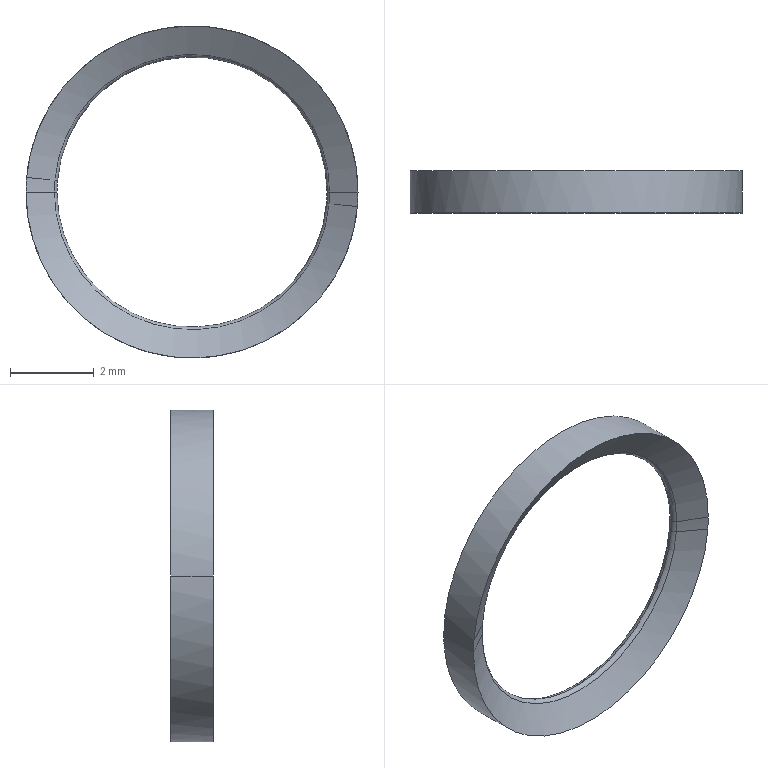Part | SolidWorks | features BaseBody 1 | 1 solid | 18 faces | box 7.92 x 1.004 x 7.92 mm | volume 9.83 mm3 | torus 8 | cone 8 | cylinder 2 | commonest cylinder face diameters 7.92 x2
STEP:
#1=CARTESIAN_POINT('',(-2079.52,1131.328,-1627.094));
#2=VERTEX_POINT('',#1);
#3=CARTESIAN_POINT('',(-2087.425,1131.328,-1627.439));
#4=VERTEX_POINT('',#3);
#5=CARTESIAN_POINT('',(-2083.48,1131.328,-1627.094));
#6=DIRECTION('',(0.,1.,0.));
#7=DIRECTION('',(1.,0.,0.));
#8=AXIS2_PLACEMENT_3D('',#5,#6,#7);
#9=CIRCLE('',#8,3.96);
#10=EDGE_CURVE('',#2,#4,#9,.T.);
#11=ORIENTED_EDGE('',*,*,#10,.F.);
#12=CARTESIAN_POINT('',(-2079.52,1130.324,-1627.094));
#13=VERTEX_POINT('',#12);
#14=CARTESIAN_POINT('',(-2079.52,1130.324,-1627.094));
#15=DIRECTION('',(0.,1.,0.));
#16=VECTOR('',#15,1000.);
#17=LINE('',#14,#16);
#18=EDGE_CURVE('',#13,#2,#17,.T.);
#19=ORIENTED_EDGE('',*,*,#18,.F.);
#20=CARTESIAN_POINT('',(-2079.536,1130.324,-1627.439));
#21=VERTEX_POINT('',#20);
#22=CARTESIAN_POINT('',(-2083.48,1130.324,-1627.094));
#23=DIRECTION('',(0.,1.,0.));
#24=DIRECTION('',(1.,0.,0.));
#25=AXIS2_PLACEMENT_3D('',#22,#23,#24);
#26=CIRCLE('',#25,3.96);
#27=EDGE_CURVE('',#13,#21,#26,.T.);
#28=ORIENTED_EDGE('',*,*,#27,.T.);
#29=CARTESIAN_POINT('',(-2087.44,1130.324,-1627.094));
#30=VERTEX_POINT('',#29);
#31=CARTESIAN_POINT('',(-2083.48,1130.324,-1627.094));
#32=DIRECTION('',(0.,1.,0.));
#33=DIRECTION('',(0.9962,0.,-0.08716));
#34=AXIS2_PLACEMENT_3D('',#31,#32,#33);
#35=CIRCLE('',#34,3.96);
#36=EDGE_CURVE('',#21,#30,#35,.T.);
#37=ORIENTED_EDGE('',*,*,#36,.T.);
#38=CARTESIAN_POINT('',(-2087.44,1131.328,-1627.094));
#39=VERTEX_POINT('',#38);
#40=CARTESIAN_POINT('',(-2087.44,1130.324,-1627.094));
#41=DIRECTION('',(0.,1.,0.));
#42=VECTOR('',#41,1000.);
#43=LINE('',#40,#42);
#44=EDGE_CURVE('',#30,#39,#43,.T.);
#45=ORIENTED_EDGE('',*,*,#44,.T.);
#46=CARTESIAN_POINT('',(-2083.48,1131.328,-1627.094));
#47=DIRECTION('',(0.,1.,0.));
#48=DIRECTION('',(-0.9962,0.,-0.08716));
#49=AXIS2_PLACEMENT_3D('',#46,#47,#48);
#50=CIRCLE('',#49,3.96);
#51=EDGE_CURVE('',#4,#39,#50,.T.);
#52=ORIENTED_EDGE('',*,*,#51,.F.);
#53=EDGE_LOOP('',(#11,#19,#28,#37,#45,#52));
#54=FACE_OUTER_BOUND('',#53,.T.);
#55=CARTESIAN_POINT('',(-2083.48,1124.59,-1627.094));
#56=DIRECTION('',(0.,1.,0.));
#57=DIRECTION('',(0.9962,0.,0.08716));
#58=AXIS2_PLACEMENT_3D('',#55,#56,#57);
#59=CYLINDRICAL_SURFACE('',#58,3.96);
#60=ADVANCED_FACE('',(#54),#59,.T.);
#61=CARTESIAN_POINT('',(-2087.425,1130.324,-1626.748));
#62=VERTEX_POINT('',#61);
#63=CARTESIAN_POINT('',(-2083.48,1130.324,-1627.094));
#64=DIRECTION('',(0.,1.,0.));
#65=DIRECTION('',(-0.9962,0.,0.08716));
#66=AXIS2_PLACEMENT_3D('',#63,#64,#65);
#67=CIRCLE('',#66,3.96);
#68=EDGE_CURVE('',#62,#13,#67,.T.);
#69=ORIENTED_EDGE('',*,*,#68,.T.);
#70=ORIENTED_EDGE('',*,*,#18,.T.);
#71=CARTESIAN_POINT('',(-2079.536,1131.328,-1626.748));
#72=VERTEX_POINT('',#71);
#73=CARTESIAN_POINT('',(-2083.48,1131.328,-1627.094));
#74=DIRECTION('',(0.,1.,0.));
#75=DIRECTION('',(0.9962,0.,0.08716));
#76=AXIS2_PLACEMENT_3D('',#73,#74,#75);
#77=CIRCLE('',#76,3.96);
#78=EDGE_CURVE('',#72,#2,#77,.T.);
#79=ORIENTED_EDGE('',*,*,#78,.F.);
#80=CARTESIAN_POINT('',(-2083.48,1131.328,-1627.094));
#81=DIRECTION('',(0.,1.,0.));
#82=DIRECTION('',(-1.,0.,0.));
#83=AXIS2_PLACEMENT_3D('',#80,#81,#82);
#84=CIRCLE('',#83,3.96);
#85=EDGE_CURVE('',#39,#72,#84,.T.);
#86=ORIENTED_EDGE('',*,*,#85,.F.);
#87=ORIENTED_EDGE('',*,*,#44,.F.);
#88=CARTESIAN_POINT('',(-2083.48,1130.324,-1627.094));
#89=DIRECTION('',(0.,1.,0.));
#90=DIRECTION('',(-1.,0.,0.));
#91=AXIS2_PLACEMENT_3D('',#88,#89,#90);
#92=CIRCLE('',#91,3.96);
#93=EDGE_CURVE('',#30,#62,#92,.T.);
#94=ORIENTED_EDGE('',*,*,#93,.T.);
#95=EDGE_LOOP('',(#69,#70,#79,#86,#87,#94));
#96=FACE_OUTER_BOUND('',#95,.T.);
#97=CARTESIAN_POINT('',(-2083.48,1124.59,-1627.094));
#98=DIRECTION('',(0.,1.,0.));
#99=DIRECTION('',(-0.9962,0.,-0.08716));
#100=AXIS2_PLACEMENT_3D('',#97,#98,#99);
#101=CYLINDRICAL_SURFACE('',#100,3.96);
#102=ADVANCED_FACE('',(#96),#101,.T.);
#103=CARTESIAN_POINT('',(-2080.207,1130.713,-1627.38));
#104=VERTEX_POINT('',#103);
#105=CARTESIAN_POINT('',(-2080.272,1130.826,-1627.374));
#106=VERTEX_POINT('',#105);
#107=CARTESIAN_POINT('',(-2080.143,1130.826,-1627.386));
#108=DIRECTION('',(-0.08716,0.,-0.9962));
#109=DIRECTION('',(-0.4981,-0.866,0.04358));
#110=AXIS2_PLACEMENT_3D('',#107,#108,#109);
#111=CIRCLE('',#110,0.1299);
#112=EDGE_CURVE('',#104,#106,#111,.T.);
#113=ORIENTED_EDGE('',*,*,#112,.T.);
#114=CARTESIAN_POINT('',(-2086.701,1130.826,-1627.094));
#115=VERTEX_POINT('',#114);
#116=CARTESIAN_POINT('',(-2083.48,1130.826,-1627.094));
#117=DIRECTION('',(0.,-1.,0.));
#118=DIRECTION('',(-1.,0.,0.));
#119=AXIS2_PLACEMENT_3D('',#116,#117,#118);
#120=CIRCLE('',#119,3.221);
#121=EDGE_CURVE('',#115,#106,#120,.T.);
#122=ORIENTED_EDGE('',*,*,#121,.F.);
#123=CARTESIAN_POINT('',(-2086.766,1130.713,-1627.094));
#124=VERTEX_POINT('',#123);
#125=CARTESIAN_POINT('',(-2086.831,1130.826,-1627.094));
#126=DIRECTION('',(0.,0.,1.));
#127=DIRECTION('',(0.5,-0.866,0.));
#128=AXIS2_PLACEMENT_3D('',#125,#126,#127);
#129=CIRCLE('',#128,0.1299);
#130=EDGE_CURVE('',#124,#115,#129,.T.);
#131=ORIENTED_EDGE('',*,*,#130,.F.);
#132=CARTESIAN_POINT('',(-2083.48,1130.713,-1627.094));
#133=DIRECTION('',(0.,-1.,0.));
#134=DIRECTION('',(-1.,0.,0.));
#135=AXIS2_PLACEMENT_3D('',#132,#133,#134);
#136=CIRCLE('',#135,3.286);
#137=EDGE_CURVE('',#124,#104,#136,.T.);
#138=ORIENTED_EDGE('',*,*,#137,.T.);
#139=EDGE_LOOP('',(#113,#122,#131,#138));
#140=FACE_OUTER_BOUND('',#139,.T.);
#141=CARTESIAN_POINT('',(-2083.48,1130.826,-1627.094));
#142=DIRECTION('',(0.,-1.,0.));
#143=DIRECTION('',(-0.9962,0.,0.08716));
#144=AXIS2_PLACEMENT_3D('',#141,#142,#143);
#145=TOROIDAL_SURFACE('',#144,3.35,0.1299);
#146=ADVANCED_FACE('',(#140),#145,.T.);
#147=CARTESIAN_POINT('',(-2086.754,1130.713,-1626.807));
#148=VERTEX_POINT('',#147);
#149=CARTESIAN_POINT('',(-2086.689,1130.826,-1626.813));
#150=VERTEX_POINT('',#149);
#151=CARTESIAN_POINT('',(-2086.818,1130.826,-1626.802));
#152=DIRECTION('',(0.08716,0.,0.9962));
#153=DIRECTION('',(0.4981,-0.866,-0.04358));
#154=AXIS2_PLACEMENT_3D('',#151,#152,#153);
#155=CIRCLE('',#154,0.1299);
#156=EDGE_CURVE('',#148,#150,#155,.T.);
#157=ORIENTED_EDGE('',*,*,#156,.T.);
#158=CARTESIAN_POINT('',(-2080.26,1130.826,-1627.094));
#159=VERTEX_POINT('',#158);
#160=CARTESIAN_POINT('',(-2083.48,1130.826,-1627.094));
#161=DIRECTION('',(0.,-1.,0.));
#162=DIRECTION('',(1.,0.,0.));
#163=AXIS2_PLACEMENT_3D('',#160,#161,#162);
#164=CIRCLE('',#163,3.221);
#165=EDGE_CURVE('',#159,#150,#164,.T.);
#166=ORIENTED_EDGE('',*,*,#165,.F.);
#167=CARTESIAN_POINT('',(-2080.195,1130.713,-1627.094));
#168=VERTEX_POINT('',#167);
#169=CARTESIAN_POINT('',(-2080.13,1130.826,-1627.094));
#170=DIRECTION('',(0.,0.,-1.));
#171=DIRECTION('',(-0.5,-0.866,0.));
#172=AXIS2_PLACEMENT_3D('',#169,#170,#171);
#173=CIRCLE('',#172,0.1299);
#174=EDGE_CURVE('',#168,#159,#173,.T.);
#175=ORIENTED_EDGE('',*,*,#174,.F.);
#176=CARTESIAN_POINT('',(-2083.48,1130.713,-1627.094));
#177=DIRECTION('',(0.,-1.,0.));
#178=DIRECTION('',(1.,0.,0.));
#179=AXIS2_PLACEMENT_3D('',#176,#177,#178);
#180=CIRCLE('',#179,3.286);
#181=EDGE_CURVE('',#168,#148,#180,.T.);
#182=ORIENTED_EDGE('',*,*,#181,.T.);
#183=EDGE_LOOP('',(#157,#166,#175,#182));
#184=FACE_OUTER_BOUND('',#183,.T.);
#185=CARTESIAN_POINT('',(-2083.48,1130.826,-1627.094));
#186=DIRECTION('',(0.,-1.,0.));
#187=DIRECTION('',(0.9962,0.,-0.08716));
#188=AXIS2_PLACEMENT_3D('',#185,#186,#187);
#189=TOROIDAL_SURFACE('',#188,3.35,0.1299);
#190=ADVANCED_FACE('',(#184),#189,.T.);
#191=CARTESIAN_POINT('',(-2086.754,1130.938,-1626.807));
#192=VERTEX_POINT('',#191);
#193=CARTESIAN_POINT('',(-2086.818,1130.826,-1626.802));
#194=DIRECTION('',(0.08716,0.,0.9962));
#195=DIRECTION('',(0.9962,0.,-0.08716));
#196=AXIS2_PLACEMENT_3D('',#193,#194,#195);
#197=CIRCLE('',#196,0.1299);
#198=EDGE_CURVE('',#150,#192,#197,.T.);
#199=ORIENTED_EDGE('',*,*,#198,.T.);
#200=CARTESIAN_POINT('',(-2080.207,1130.938,-1626.807));
#201=VERTEX_POINT('',#200);
#202=CARTESIAN_POINT('',(-2083.48,1130.938,-1627.094));
#203=DIRECTION('',(0.,-1.,0.));
#204=DIRECTION('',(0.9962,0.,0.08716));
#205=AXIS2_PLACEMENT_3D('',#202,#203,#204);
#206=CIRCLE('',#205,3.286);
#207=EDGE_CURVE('',#201,#192,#206,.T.);
#208=ORIENTED_EDGE('',*,*,#207,.F.);
#209=CARTESIAN_POINT('',(-2080.195,1130.938,-1627.094));
#210=VERTEX_POINT('',#209);
#211=CARTESIAN_POINT('',(-2083.48,1130.938,-1627.094));
#212=DIRECTION('',(0.,-1.,0.));
#213=DIRECTION('',(1.,0.,0.));
#214=AXIS2_PLACEMENT_3D('',#211,#212,#213);
#215=CIRCLE('',#214,3.286);
#216=EDGE_CURVE('',#210,#201,#215,.T.);
#217=ORIENTED_EDGE('',*,*,#216,.F.);
#218=CARTESIAN_POINT('',(-2080.13,1130.826,-1627.094));
#219=DIRECTION('',(0.,0.,-1.));
#220=DIRECTION('',(-1.,0.,0.));
#221=AXIS2_PLACEMENT_3D('',#218,#219,#220);
#222=CIRCLE('',#221,0.1299);
#223=EDGE_CURVE('',#159,#210,#222,.T.);
#224=ORIENTED_EDGE('',*,*,#223,.F.);
#225=ORIENTED_EDGE('',*,*,#165,.T.);
#226=EDGE_LOOP('',(#199,#208,#217,#224,#225));
#227=FACE_OUTER_BOUND('',#226,.T.);
#228=CARTESIAN_POINT('',(-2083.48,1130.826,-1627.094));
#229=DIRECTION('',(0.,-1.,0.));
#230=DIRECTION('',(0.9962,0.,-0.08716));
#231=AXIS2_PLACEMENT_3D('',#228,#229,#230);
#232=TOROIDAL_SURFACE('',#231,3.35,0.1299);
#233=ADVANCED_FACE('',(#227),#232,.T.);
#234=CARTESIAN_POINT('',(-2086.754,1130.938,-1627.38));
#235=VERTEX_POINT('',#234);
#236=CARTESIAN_POINT('',(-2087.425,1131.328,-1627.439));
#237=DIRECTION('',(0.8627,-0.5,0.07548));
#238=VECTOR('',#237,1000.);
#239=LINE('',#236,#238);
#240=EDGE_CURVE('',#4,#235,#239,.T.);
#241=ORIENTED_EDGE('',*,*,#240,.T.);
#242=CARTESIAN_POINT('',(-2080.207,1130.938,-1627.38));
#243=VERTEX_POINT('',#242);
#244=CARTESIAN_POINT('',(-2083.48,1130.938,-1627.094));
#245=DIRECTION('',(0.,-1.,0.));
#246=DIRECTION('',(-0.9962,0.,-0.08716));
#247=AXIS2_PLACEMENT_3D('',#244,#245,#246);
#248=CIRCLE('',#247,3.286);
#249=EDGE_CURVE('',#235,#243,#248,.T.);
#250=ORIENTED_EDGE('',*,*,#249,.T.);
#251=CARTESIAN_POINT('',(-2083.48,1130.938,-1627.094));
#252=DIRECTION('',(0.,-1.,0.));
#253=DIRECTION('',(0.9962,0.,-0.08716));
#254=AXIS2_PLACEMENT_3D('',#251,#252,#253);
#255=CIRCLE('',#254,3.286);
#256=EDGE_CURVE('',#243,#210,#255,.T.);
#257=ORIENTED_EDGE('',*,*,#256,.T.);
#258=CARTESIAN_POINT('',(-2080.195,1130.938,-1627.094));
#259=DIRECTION('',(0.866,0.5,0.));
#260=VECTOR('',#259,1000.);
#261=LINE('',#258,#260);
#262=EDGE_CURVE('',#210,#2,#261,.T.);
#263=ORIENTED_EDGE('',*,*,#262,.T.);
#264=ORIENTED_EDGE('',*,*,#10,.T.);
#265=EDGE_LOOP('',(#241,#250,#257,#263,#264));
#266=FACE_OUTER_BOUND('',#265,.T.);
#267=CARTESIAN_POINT('',(-2083.48,1130.918,-1627.094));
#268=DIRECTION('',(0.,1.,0.));
#269=DIRECTION('',(0.9962,0.,0.08716));
#270=AXIS2_PLACEMENT_3D('',#267,#268,#269);
#271=CONICAL_SURFACE('',#270,3.25,1.047);
#272=ADVANCED_FACE('',(#266),#271,.F.);
#273=CARTESIAN_POINT('',(-2079.536,1130.324,-1627.439));
#274=DIRECTION('',(-0.8627,0.5,0.07548));
#275=VECTOR('',#274,1000.);
#276=LINE('',#273,#275);
#277=EDGE_CURVE('',#21,#104,#276,.T.);
#278=ORIENTED_EDGE('',*,*,#277,.T.);
#279=ORIENTED_EDGE('',*,*,#137,.F.);
#280=CARTESIAN_POINT('',(-2086.766,1130.713,-1627.094));
#281=DIRECTION('',(-0.866,-0.5,0.));
#282=VECTOR('',#281,1000.);
#283=LINE('',#280,#282);
#284=EDGE_CURVE('',#124,#30,#283,.T.);
#285=ORIENTED_EDGE('',*,*,#284,.T.);
#286=ORIENTED_EDGE('',*,*,#36,.F.);
#287=EDGE_LOOP('',(#278,#279,#285,#286));
#288=FACE_OUTER_BOUND('',#287,.T.);
#289=CARTESIAN_POINT('',(-2083.48,1130.734,-1627.094));
#290=DIRECTION('',(0.,-1.,0.));
#291=DIRECTION('',(-0.9962,0.,0.08716));
#292=AXIS2_PLACEMENT_3D('',#289,#290,#291);
#293=CONICAL_SURFACE('',#292,3.25,1.047);
#294=ADVANCED_FACE('',(#288),#293,.F.);
#295=CARTESIAN_POINT('',(-2087.425,1130.324,-1626.748));
#296=DIRECTION('',(0.8627,0.5,-0.07548));
#297=VECTOR('',#296,1000.);
#298=LINE('',#295,#297);
#299=EDGE_CURVE('',#62,#148,#298,.T.);
#300=ORIENTED_EDGE('',*,*,#299,.T.);
#301=ORIENTED_EDGE('',*,*,#181,.F.);
#302=CARTESIAN_POINT('',(-2080.195,1130.713,-1627.094));
#303=DIRECTION('',(0.866,-0.5,0.));
#304=VECTOR('',#303,1000.);
#305=LINE('',#302,#304);
#306=EDGE_CURVE('',#168,#13,#305,.T.);
#307=ORIENTED_EDGE('',*,*,#306,.T.);
#308=ORIENTED_EDGE('',*,*,#68,.F.);
#309=EDGE_LOOP('',(#300,#301,#307,#308));
#310=FACE_OUTER_BOUND('',#309,.T.);
#311=CARTESIAN_POINT('',(-2083.48,1130.734,-1627.094));
#312=DIRECTION('',(0.,-1.,0.));
#313=DIRECTION('',(0.9962,0.,-0.08716));
#314=AXIS2_PLACEMENT_3D('',#311,#312,#313);
#315=CONICAL_SURFACE('',#314,3.25,1.047);
#316=ADVANCED_FACE('',(#310),#315,.F.);
#317=CARTESIAN_POINT('',(-2079.536,1131.328,-1626.748));
#318=DIRECTION('',(-0.8627,-0.5,-0.07548));
#319=VECTOR('',#318,1000.);
#320=LINE('',#317,#319);
#321=EDGE_CURVE('',#72,#201,#320,.T.);
#322=ORIENTED_EDGE('',*,*,#321,.T.);
#323=ORIENTED_EDGE('',*,*,#207,.T.);
#324=CARTESIAN_POINT('',(-2086.766,1130.938,-1627.094));
#325=VERTEX_POINT('',#324);
#326=CARTESIAN_POINT('',(-2083.48,1130.938,-1627.094));
#327=DIRECTION('',(0.,-1.,0.));
#328=DIRECTION('',(-0.9962,0.,0.08716));
#329=AXIS2_PLACEMENT_3D('',#326,#327,#328);
#330=CIRCLE('',#329,3.286);
#331=EDGE_CURVE('',#192,#325,#330,.T.);
#332=ORIENTED_EDGE('',*,*,#331,.T.);
#333=CARTESIAN_POINT('',(-2086.766,1130.938,-1627.094));
#334=DIRECTION('',(-0.866,0.5,0.));
#335=VECTOR('',#334,1000.);
#336=LINE('',#333,#335);
#337=EDGE_CURVE('',#325,#39,#336,.T.);
#338=ORIENTED_EDGE('',*,*,#337,.T.);
#339=ORIENTED_EDGE('',*,*,#85,.T.);
#340=EDGE_LOOP('',(#322,#323,#332,#338,#339));
#341=FACE_OUTER_BOUND('',#340,.T.);
#342=CARTESIAN_POINT('',(-2083.48,1130.918,-1627.094));
#343=DIRECTION('',(0.,1.,0.));
#344=DIRECTION('',(-0.9962,0.,-0.08716));
#345=AXIS2_PLACEMENT_3D('',#342,#343,#344);
#346=CONICAL_SURFACE('',#345,3.25,1.047);
#347=ADVANCED_FACE('',(#341),#346,.F.);
#348=CARTESIAN_POINT('',(-2080.143,1130.826,-1627.386));
#349=DIRECTION('',(-0.08716,0.,-0.9962));
#350=DIRECTION('',(-0.9962,0.,0.08716));
#351=AXIS2_PLACEMENT_3D('',#348,#349,#350);
#352=CIRCLE('',#351,0.1299);
#353=EDGE_CURVE('',#106,#243,#352,.T.);
#354=ORIENTED_EDGE('',*,*,#353,.T.);
#355=ORIENTED_EDGE('',*,*,#249,.F.);
#356=CARTESIAN_POINT('',(-2083.48,1130.938,-1627.094));
#357=DIRECTION('',(0.,-1.,0.));
#358=DIRECTION('',(-1.,0.,0.));
#359=AXIS2_PLACEMENT_3D('',#356,#357,#358);
#360=CIRCLE('',#359,3.286);
#361=EDGE_CURVE('',#325,#235,#360,.T.);
#362=ORIENTED_EDGE('',*,*,#361,.F.);
#363=CARTESIAN_POINT('',(-2086.831,1130.826,-1627.094));
#364=DIRECTION('',(0.,0.,1.));
#365=DIRECTION('',(1.,0.,0.));
#366=AXIS2_PLACEMENT_3D('',#363,#364,#365);
#367=CIRCLE('',#366,0.1299);
#368=EDGE_CURVE('',#115,#325,#367,.T.);
#369=ORIENTED_EDGE('',*,*,#368,.F.);
#370=ORIENTED_EDGE('',*,*,#121,.T.);
#371=EDGE_LOOP('',(#354,#355,#362,#369,#370));
#372=FACE_OUTER_BOUND('',#371,.T.);
#373=CARTESIAN_POINT('',(-2083.48,1130.826,-1627.094));
#374=DIRECTION('',(0.,-1.,0.));
#375=DIRECTION('',(-0.9962,0.,0.08716));
#376=AXIS2_PLACEMENT_3D('',#373,#374,#375);
#377=TOROIDAL_SURFACE('',#376,3.35,0.1299);
#378=ADVANCED_FACE('',(#372),#377,.T.);
#379=ORIENTED_EDGE('',*,*,#353,.F.);
#380=CARTESIAN_POINT('',(-2083.48,1130.826,-1627.094));
#381=DIRECTION('',(0.,-1.,0.));
#382=DIRECTION('',(0.9962,0.,-0.08716));
#383=AXIS2_PLACEMENT_3D('',#380,#381,#382);
#384=CIRCLE('',#383,3.221);
#385=EDGE_CURVE('',#106,#159,#384,.T.);
#386=ORIENTED_EDGE('',*,*,#385,.T.);
#387=ORIENTED_EDGE('',*,*,#223,.T.);
#388=ORIENTED_EDGE('',*,*,#256,.F.);
#389=EDGE_LOOP('',(#379,#386,#387,#388));
#390=FACE_OUTER_BOUND('',#389,.T.);
#391=CARTESIAN_POINT('',(-2083.48,1130.826,-1627.094));
#392=DIRECTION('',(0.,-1.,0.));
#393=DIRECTION('',(0.9848,0.,-0.1736));
#394=AXIS2_PLACEMENT_3D('',#391,#392,#393);
#395=TOROIDAL_SURFACE('',#394,3.35,0.1299);
#396=ADVANCED_FACE('',(#390),#395,.T.);
#397=ORIENTED_EDGE('',*,*,#78,.T.);
#398=ORIENTED_EDGE('',*,*,#262,.F.);
#399=ORIENTED_EDGE('',*,*,#216,.T.);
#400=ORIENTED_EDGE('',*,*,#321,.F.);
#401=EDGE_LOOP('',(#397,#398,#399,#400));
#402=FACE_OUTER_BOUND('',#401,.T.);
#403=CARTESIAN_POINT('',(-2083.48,1130.918,-1627.094));
#404=DIRECTION('',(0.,1.,0.));
#405=DIRECTION('',(0.9848,0.,0.1736));
#406=AXIS2_PLACEMENT_3D('',#403,#404,#405);
#407=CONICAL_SURFACE('',#406,3.25,1.047);
#408=ADVANCED_FACE('',(#402),#407,.F.);
#409=ORIENTED_EDGE('',*,*,#93,.F.);
#410=ORIENTED_EDGE('',*,*,#284,.F.);
#411=CARTESIAN_POINT('',(-2083.48,1130.713,-1627.094));
#412=DIRECTION('',(0.,-1.,0.));
#413=DIRECTION('',(-0.9962,0.,0.08716));
#414=AXIS2_PLACEMENT_3D('',#411,#412,#413);
#415=CIRCLE('',#414,3.286);
#416=EDGE_CURVE('',#148,#124,#415,.T.);
#417=ORIENTED_EDGE('',*,*,#416,.F.);
#418=ORIENTED_EDGE('',*,*,#299,.F.);
#419=EDGE_LOOP('',(#409,#410,#417,#418));
#420=FACE_OUTER_BOUND('',#419,.T.);
#421=CARTESIAN_POINT('',(-2083.48,1130.734,-1627.094));
#422=DIRECTION('',(0.,-1.,0.));
#423=DIRECTION('',(-0.9848,0.,0.1736));
#424=AXIS2_PLACEMENT_3D('',#421,#422,#423);
#425=CONICAL_SURFACE('',#424,3.25,1.047);
#426=ADVANCED_FACE('',(#420),#425,.F.);
#427=ORIENTED_EDGE('',*,*,#27,.F.);
#428=ORIENTED_EDGE('',*,*,#306,.F.);
#429=CARTESIAN_POINT('',(-2083.48,1130.713,-1627.094));
#430=DIRECTION('',(0.,-1.,0.));
#431=DIRECTION('',(0.9962,0.,-0.08716));
#432=AXIS2_PLACEMENT_3D('',#429,#430,#431);
#433=CIRCLE('',#432,3.286);
#434=EDGE_CURVE('',#104,#168,#433,.T.);
#435=ORIENTED_EDGE('',*,*,#434,.F.);
#436=ORIENTED_EDGE('',*,*,#277,.F.);
#437=EDGE_LOOP('',(#427,#428,#435,#436));
#438=FACE_OUTER_BOUND('',#437,.T.);
#439=CARTESIAN_POINT('',(-2083.48,1130.734,-1627.094));
#440=DIRECTION('',(0.,-1.,0.));
#441=DIRECTION('',(0.9848,0.,-0.1736));
#442=AXIS2_PLACEMENT_3D('',#439,#440,#441);
#443=CONICAL_SURFACE('',#442,3.25,1.047);
#444=ADVANCED_FACE('',(#438),#443,.F.);
#445=ORIENTED_EDGE('',*,*,#51,.T.);
#446=ORIENTED_EDGE('',*,*,#337,.F.);
#447=ORIENTED_EDGE('',*,*,#361,.T.);
#448=ORIENTED_EDGE('',*,*,#240,.F.);
#449=EDGE_LOOP('',(#445,#446,#447,#448));
#450=FACE_OUTER_BOUND('',#449,.T.);
#451=CARTESIAN_POINT('',(-2083.48,1130.918,-1627.094));
#452=DIRECTION('',(0.,1.,0.));
#453=DIRECTION('',(-0.9848,0.,-0.1736));
#454=AXIS2_PLACEMENT_3D('',#451,#452,#453);
#455=CONICAL_SURFACE('',#454,3.25,1.047);
#456=ADVANCED_FACE('',(#450),#455,.F.);
#457=ORIENTED_EDGE('',*,*,#198,.F.);
#458=CARTESIAN_POINT('',(-2083.48,1130.826,-1627.094));
#459=DIRECTION('',(0.,-1.,0.));
#460=DIRECTION('',(-0.9962,0.,0.08716));
#461=AXIS2_PLACEMENT_3D('',#458,#459,#460);
#462=CIRCLE('',#461,3.221);
#463=EDGE_CURVE('',#150,#115,#462,.T.);
#464=ORIENTED_EDGE('',*,*,#463,.T.);
#465=ORIENTED_EDGE('',*,*,#368,.T.);
#466=ORIENTED_EDGE('',*,*,#331,.F.);
#467=EDGE_LOOP('',(#457,#464,#465,#466));
#468=FACE_OUTER_BOUND('',#467,.T.);
#469=CARTESIAN_POINT('',(-2083.48,1130.826,-1627.094));
#470=DIRECTION('',(0.,-1.,0.));
#471=DIRECTION('',(-0.9848,0.,0.1736));
#472=AXIS2_PLACEMENT_3D('',#469,#470,#471);
#473=TOROIDAL_SURFACE('',#472,3.35,0.1299);
#474=ADVANCED_FACE('',(#468),#473,.T.);
#475=ORIENTED_EDGE('',*,*,#156,.F.);
#476=ORIENTED_EDGE('',*,*,#416,.T.);
#477=ORIENTED_EDGE('',*,*,#130,.T.);
#478=ORIENTED_EDGE('',*,*,#463,.F.);
#479=EDGE_LOOP('',(#475,#476,#477,#478));
#480=FACE_OUTER_BOUND('',#479,.T.);
#481=CARTESIAN_POINT('',(-2083.48,1130.826,-1627.094));
#482=DIRECTION('',(0.,-1.,0.));
#483=DIRECTION('',(-0.9848,0.,0.1736));
#484=AXIS2_PLACEMENT_3D('',#481,#482,#483);
#485=TOROIDAL_SURFACE('',#484,3.35,0.1299);
#486=ADVANCED_FACE('',(#480),#485,.T.);
#487=ORIENTED_EDGE('',*,*,#112,.F.);
#488=ORIENTED_EDGE('',*,*,#434,.T.);
#489=ORIENTED_EDGE('',*,*,#174,.T.);
#490=ORIENTED_EDGE('',*,*,#385,.F.);
#491=EDGE_LOOP('',(#487,#488,#489,#490));
#492=FACE_OUTER_BOUND('',#491,.T.);
#493=CARTESIAN_POINT('',(-2083.48,1130.826,-1627.094));
#494=DIRECTION('',(0.,-1.,0.));
#495=DIRECTION('',(0.9848,0.,-0.1736));
#496=AXIS2_PLACEMENT_3D('',#493,#494,#495);
#497=TOROIDAL_SURFACE('',#496,3.35,0.1299);
#498=ADVANCED_FACE('',(#492),#497,.T.);
#499=CLOSED_SHELL('',(#60,#102,#146,#190,#233,#272,#294,#316,#347,#378,#396,#408,#426,#444,#456,#474,#486,#498));
#500=MANIFOLD_SOLID_BREP('',#499);
#501=CARTESIAN_POINT('',(0.,0.,0.));
#502=DIRECTION('',(0.,0.,1.));
#503=DIRECTION('',(1.,0.,0.));
#504=AXIS2_PLACEMENT_3D('',#501,#502,#503);
#505=(LENGTH_UNIT()NAMED_UNIT(*)SI_UNIT(.MILLI.,.METRE.));
#506=UNCERTAINTY_MEASURE_WITH_UNIT(LENGTH_MEASURE(0.00001),#505,'','');
#507=(NAMED_UNIT(*)PLANE_ANGLE_UNIT()SI_UNIT($,.RADIAN.));
#508=(NAMED_UNIT(*)SI_UNIT($,.STERADIAN.)SOLID_ANGLE_UNIT());
#509=(GEOMETRIC_REPRESENTATION_CONTEXT(3)GLOBAL_UNCERTAINTY_ASSIGNED_CONTEXT((#506))GLOBAL_UNIT_ASSIGNED_CONTEXT((#505,#507,#508))REPRESENTATION_CONTEXT('',''));
#510=ADVANCED_BREP_SHAPE_REPRESENTATION('',(#500,#504),#509);